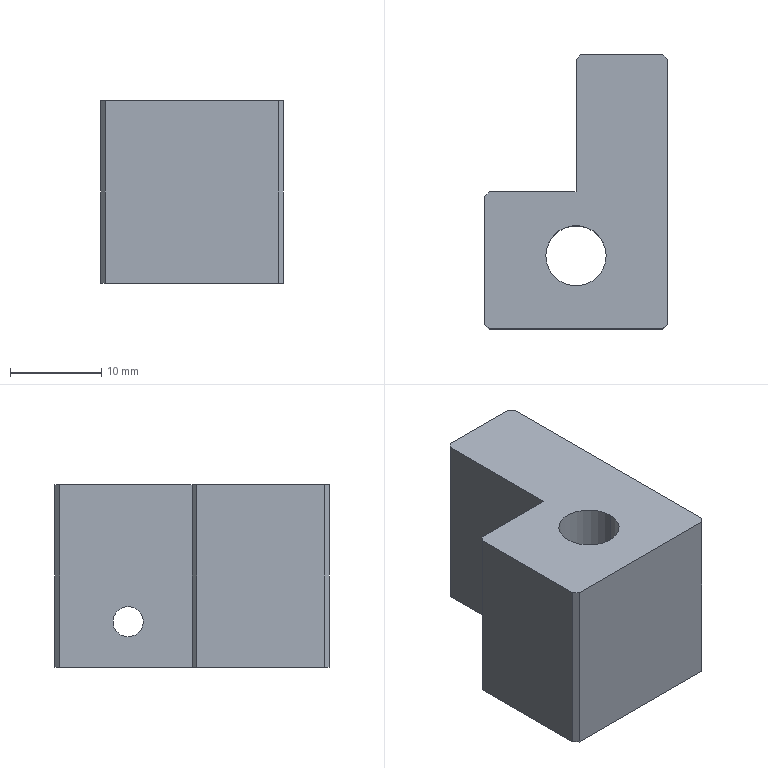Part | SolidWorks | features HoleWzd 2, Chamfer 1, Extrusion 1, ICE 1 | 1 solid | 20 faces | box 20 x 30 x 20 mm | volume 7804 mm3 | plane 14 | cylinder 6 | commonest cylinder face diameters 3.3 x2 6.6 x2 11 x2
STEP:
#1=CARTESIAN_POINT('',(10.,7.,3.35));
#2=VERTEX_POINT('',#1);
#3=CARTESIAN_POINT('',(10.,7.,6.65));
#4=VERTEX_POINT('',#3);
#5=CARTESIAN_POINT('',(10.,7.,5.));
#6=DIRECTION('',(-1.,0.,0.));
#7=DIRECTION('',(0.,0.,1.));
#8=AXIS2_PLACEMENT_3D('',#5,#6,#7);
#9=CIRCLE('',#8,1.65);
#10=EDGE_CURVE('',#2,#4,#9,.T.);
#11=ORIENTED_EDGE('',*,*,#10,.F.);
#12=CARTESIAN_POINT('',(0.,7.,3.35));
#13=VERTEX_POINT('',#12);
#14=CARTESIAN_POINT('',(0.,7.,3.35));
#15=DIRECTION('',(-1.,0.,0.));
#16=VECTOR('',#15,1000.);
#17=LINE('',#14,#16);
#18=EDGE_CURVE('',#2,#13,#17,.T.);
#19=ORIENTED_EDGE('',*,*,#18,.T.);
#20=CARTESIAN_POINT('',(0.,7.,6.65));
#21=VERTEX_POINT('',#20);
#22=CARTESIAN_POINT('',(0.,7.,5.));
#23=DIRECTION('',(-1.,0.,0.));
#24=DIRECTION('',(0.,0.,1.));
#25=AXIS2_PLACEMENT_3D('',#22,#23,#24);
#26=CIRCLE('',#25,1.65);
#27=EDGE_CURVE('',#13,#21,#26,.T.);
#28=ORIENTED_EDGE('',*,*,#27,.T.);
#29=CARTESIAN_POINT('',(0.,7.,6.65));
#30=DIRECTION('',(-1.,0.,0.));
#31=VECTOR('',#30,1000.);
#32=LINE('',#29,#31);
#33=EDGE_CURVE('',#4,#21,#32,.T.);
#34=ORIENTED_EDGE('',*,*,#33,.F.);
#35=EDGE_LOOP('',(#11,#19,#28,#34));
#36=FACE_OUTER_BOUND('',#35,.T.);
#37=CARTESIAN_POINT('',(0.,7.,5.));
#38=DIRECTION('',(-1.,0.,0.));
#39=DIRECTION('',(0.,0.,1.));
#40=AXIS2_PLACEMENT_3D('',#37,#38,#39);
#41=CYLINDRICAL_SURFACE('',#40,1.65);
#42=ADVANCED_FACE('',(#36),#41,.F.);
#43=CARTESIAN_POINT('',(5.5,-7.,6.8));
#44=VERTEX_POINT('',#43);
#45=CARTESIAN_POINT('',(-5.5,-7.,6.8));
#46=VERTEX_POINT('',#45);
#47=CARTESIAN_POINT('',(0.,-7.,6.8));
#48=DIRECTION('',(0.,0.,-1.));
#49=DIRECTION('',(-1.,0.,0.));
#50=AXIS2_PLACEMENT_3D('',#47,#48,#49);
#51=CIRCLE('',#50,5.5);
#52=EDGE_CURVE('',#44,#46,#51,.T.);
#53=ORIENTED_EDGE('',*,*,#52,.F.);
#54=CARTESIAN_POINT('',(5.5,-7.,0.));
#55=VERTEX_POINT('',#54);
#56=CARTESIAN_POINT('',(5.5,-7.,0.));
#57=DIRECTION('',(0.,0.,-1.));
#58=VECTOR('',#57,1000.);
#59=LINE('',#56,#58);
#60=EDGE_CURVE('',#44,#55,#59,.T.);
#61=ORIENTED_EDGE('',*,*,#60,.T.);
#62=CARTESIAN_POINT('',(-5.5,-7.,0.));
#63=VERTEX_POINT('',#62);
#64=CARTESIAN_POINT('',(0.,-7.,0.));
#65=DIRECTION('',(0.,0.,-1.));
#66=DIRECTION('',(-1.,0.,0.));
#67=AXIS2_PLACEMENT_3D('',#64,#65,#66);
#68=CIRCLE('',#67,5.5);
#69=EDGE_CURVE('',#55,#63,#68,.T.);
#70=ORIENTED_EDGE('',*,*,#69,.T.);
#71=CARTESIAN_POINT('',(-5.5,-7.,0.));
#72=DIRECTION('',(0.,0.,-1.));
#73=VECTOR('',#72,1000.);
#74=LINE('',#71,#73);
#75=EDGE_CURVE('',#46,#63,#74,.T.);
#76=ORIENTED_EDGE('',*,*,#75,.F.);
#77=EDGE_LOOP('',(#53,#61,#70,#76));
#78=FACE_OUTER_BOUND('',#77,.T.);
#79=CARTESIAN_POINT('',(0.,-7.,0.));
#80=DIRECTION('',(0.,0.,-1.));
#81=DIRECTION('',(-1.,0.,0.));
#82=AXIS2_PLACEMENT_3D('',#79,#80,#81);
#83=CYLINDRICAL_SURFACE('',#82,5.5);
#84=ADVANCED_FACE('',(#78),#83,.F.);
#85=CARTESIAN_POINT('',(3.3,-7.,20.));
#86=VERTEX_POINT('',#85);
#87=CARTESIAN_POINT('',(-3.3,-7.,20.));
#88=VERTEX_POINT('',#87);
#89=CARTESIAN_POINT('',(0.,-7.,20.));
#90=DIRECTION('',(0.,0.,-1.));
#91=DIRECTION('',(-1.,0.,0.));
#92=AXIS2_PLACEMENT_3D('',#89,#90,#91);
#93=CIRCLE('',#92,3.3);
#94=EDGE_CURVE('',#86,#88,#93,.T.);
#95=ORIENTED_EDGE('',*,*,#94,.F.);
#96=CARTESIAN_POINT('',(3.3,-7.,6.8));
#97=VERTEX_POINT('',#96);
#98=CARTESIAN_POINT('',(3.3,-7.,0.));
#99=DIRECTION('',(0.,0.,-1.));
#100=VECTOR('',#99,1000.);
#101=LINE('',#98,#100);
#102=EDGE_CURVE('',#86,#97,#101,.T.);
#103=ORIENTED_EDGE('',*,*,#102,.T.);
#104=CARTESIAN_POINT('',(-3.3,-7.,6.8));
#105=VERTEX_POINT('',#104);
#106=CARTESIAN_POINT('',(0.,-7.,6.8));
#107=DIRECTION('',(0.,0.,-1.));
#108=DIRECTION('',(-1.,0.,0.));
#109=AXIS2_PLACEMENT_3D('',#106,#107,#108);
#110=CIRCLE('',#109,3.3);
#111=EDGE_CURVE('',#97,#105,#110,.T.);
#112=ORIENTED_EDGE('',*,*,#111,.T.);
#113=CARTESIAN_POINT('',(-3.3,-7.,0.));
#114=DIRECTION('',(0.,0.,-1.));
#115=VECTOR('',#114,1000.);
#116=LINE('',#113,#115);
#117=EDGE_CURVE('',#88,#105,#116,.T.);
#118=ORIENTED_EDGE('',*,*,#117,.F.);
#119=EDGE_LOOP('',(#95,#103,#112,#118));
#120=FACE_OUTER_BOUND('',#119,.T.);
#121=CARTESIAN_POINT('',(0.,-7.,0.));
#122=DIRECTION('',(0.,0.,-1.));
#123=DIRECTION('',(-1.,0.,0.));
#124=AXIS2_PLACEMENT_3D('',#121,#122,#123);
#125=CYLINDRICAL_SURFACE('',#124,3.3);
#126=ADVANCED_FACE('',(#120),#125,.F.);
#127=CARTESIAN_POINT('',(10.,7.,5.));
#128=DIRECTION('',(-1.,0.,0.));
#129=DIRECTION('',(0.,0.,1.));
#130=AXIS2_PLACEMENT_3D('',#127,#128,#129);
#131=CIRCLE('',#130,1.65);
#132=EDGE_CURVE('',#4,#2,#131,.T.);
#133=ORIENTED_EDGE('',*,*,#132,.T.);
#134=ORIENTED_EDGE('',*,*,#10,.T.);
#135=EDGE_LOOP('',(#133,#134));
#136=FACE_BOUND('',#135,.T.);
#137=CARTESIAN_POINT('',(10.,-14.5,0.));
#138=VERTEX_POINT('',#137);
#139=CARTESIAN_POINT('',(10.,14.5,0.));
#140=VERTEX_POINT('',#139);
#141=CARTESIAN_POINT('',(10.,15.,0.));
#142=DIRECTION('',(0.,1.,0.));
#143=VECTOR('',#142,1000.);
#144=LINE('',#141,#143);
#145=EDGE_CURVE('',#138,#140,#144,.T.);
#146=ORIENTED_EDGE('',*,*,#145,.T.);
#147=CARTESIAN_POINT('',(10.,14.5,20.));
#148=VERTEX_POINT('',#147);
#149=CARTESIAN_POINT('',(10.,14.5,20.));
#150=DIRECTION('',(0.,0.,1.));
#151=VECTOR('',#150,1000.);
#152=LINE('',#149,#151);
#153=EDGE_CURVE('',#140,#148,#152,.T.);
#154=ORIENTED_EDGE('',*,*,#153,.T.);
#155=CARTESIAN_POINT('',(10.,-14.5,20.));
#156=VERTEX_POINT('',#155);
#157=CARTESIAN_POINT('',(10.,15.,20.));
#158=DIRECTION('',(0.,1.,0.));
#159=VECTOR('',#158,1000.);
#160=LINE('',#157,#159);
#161=EDGE_CURVE('',#156,#148,#160,.T.);
#162=ORIENTED_EDGE('',*,*,#161,.F.);
#163=CARTESIAN_POINT('',(10.,-14.5,20.));
#164=DIRECTION('',(0.,0.,-1.));
#165=VECTOR('',#164,1000.);
#166=LINE('',#163,#165);
#167=EDGE_CURVE('',#156,#138,#166,.T.);
#168=ORIENTED_EDGE('',*,*,#167,.T.);
#169=EDGE_LOOP('',(#146,#154,#162,#168));
#170=FACE_OUTER_BOUND('',#169,.T.);
#171=CARTESIAN_POINT('',(10.,15.,20.));
#172=DIRECTION('',(-1.,0.,0.));
#173=DIRECTION('',(0.,-1.,0.));
#174=AXIS2_PLACEMENT_3D('',#171,#172,#173);
#175=PLANE('',#174);
#176=ADVANCED_FACE('',(#136,#170),#175,.F.);
#177=CARTESIAN_POINT('',(9.5,15.,20.));
#178=VERTEX_POINT('',#177);
#179=CARTESIAN_POINT('',(0.5,15.,20.));
#180=VERTEX_POINT('',#179);
#181=CARTESIAN_POINT('',(-10.,15.,20.));
#182=DIRECTION('',(-1.,0.,0.));
#183=VECTOR('',#182,1000.);
#184=LINE('',#181,#183);
#185=EDGE_CURVE('',#178,#180,#184,.T.);
#186=ORIENTED_EDGE('',*,*,#185,.F.);
#187=CARTESIAN_POINT('',(9.5,15.,0.));
#188=VERTEX_POINT('',#187);
#189=CARTESIAN_POINT('',(9.5,15.,20.));
#190=DIRECTION('',(0.,0.,-1.));
#191=VECTOR('',#190,1000.);
#192=LINE('',#189,#191);
#193=EDGE_CURVE('',#178,#188,#192,.T.);
#194=ORIENTED_EDGE('',*,*,#193,.T.);
#195=CARTESIAN_POINT('',(0.5,15.,0.));
#196=VERTEX_POINT('',#195);
#197=CARTESIAN_POINT('',(-10.,15.,0.));
#198=DIRECTION('',(-1.,0.,0.));
#199=VECTOR('',#198,1000.);
#200=LINE('',#197,#199);
#201=EDGE_CURVE('',#188,#196,#200,.T.);
#202=ORIENTED_EDGE('',*,*,#201,.T.);
#203=CARTESIAN_POINT('',(0.5,15.,20.));
#204=DIRECTION('',(0.,0.,1.));
#205=VECTOR('',#204,1000.);
#206=LINE('',#203,#205);
#207=EDGE_CURVE('',#196,#180,#206,.T.);
#208=ORIENTED_EDGE('',*,*,#207,.T.);
#209=EDGE_LOOP('',(#186,#194,#202,#208));
#210=FACE_OUTER_BOUND('',#209,.T.);
#211=CARTESIAN_POINT('',(-10.,15.,20.));
#212=DIRECTION('',(0.,-1.,0.));
#213=DIRECTION('',(0.,0.,-1.));
#214=AXIS2_PLACEMENT_3D('',#211,#212,#213);
#215=PLANE('',#214);
#216=ADVANCED_FACE('',(#210),#215,.F.);
#217=CARTESIAN_POINT('',(-10.,-0.5,20.));
#218=VERTEX_POINT('',#217);
#219=CARTESIAN_POINT('',(-10.,-14.5,20.));
#220=VERTEX_POINT('',#219);
#221=CARTESIAN_POINT('',(-10.,15.,20.));
#222=DIRECTION('',(0.,-1.,0.));
#223=VECTOR('',#222,1000.);
#224=LINE('',#221,#223);
#225=EDGE_CURVE('',#218,#220,#224,.T.);
#226=ORIENTED_EDGE('',*,*,#225,.F.);
#227=CARTESIAN_POINT('',(-10.,-0.5,0.));
#228=VERTEX_POINT('',#227);
#229=CARTESIAN_POINT('',(-10.,-0.5,20.));
#230=DIRECTION('',(0.,0.,-1.));
#231=VECTOR('',#230,1000.);
#232=LINE('',#229,#231);
#233=EDGE_CURVE('',#218,#228,#232,.T.);
#234=ORIENTED_EDGE('',*,*,#233,.T.);
#235=CARTESIAN_POINT('',(-10.,-14.5,0.));
#236=VERTEX_POINT('',#235);
#237=CARTESIAN_POINT('',(-10.,15.,0.));
#238=DIRECTION('',(0.,-1.,0.));
#239=VECTOR('',#238,1000.);
#240=LINE('',#237,#239);
#241=EDGE_CURVE('',#228,#236,#240,.T.);
#242=ORIENTED_EDGE('',*,*,#241,.T.);
#243=CARTESIAN_POINT('',(-10.,-14.5,20.));
#244=DIRECTION('',(0.,0.,1.));
#245=VECTOR('',#244,1000.);
#246=LINE('',#243,#245);
#247=EDGE_CURVE('',#236,#220,#246,.T.);
#248=ORIENTED_EDGE('',*,*,#247,.T.);
#249=EDGE_LOOP('',(#226,#234,#242,#248));
#250=FACE_OUTER_BOUND('',#249,.T.);
#251=CARTESIAN_POINT('',(-10.,15.,20.));
#252=DIRECTION('',(1.,0.,0.));
#253=DIRECTION('',(0.,1.,0.));
#254=AXIS2_PLACEMENT_3D('',#251,#252,#253);
#255=PLANE('',#254);
#256=ADVANCED_FACE('',(#250),#255,.F.);
#257=CARTESIAN_POINT('',(-9.5,-15.,20.));
#258=VERTEX_POINT('',#257);
#259=CARTESIAN_POINT('',(9.5,-15.,20.));
#260=VERTEX_POINT('',#259);
#261=CARTESIAN_POINT('',(-10.,-15.,20.));
#262=DIRECTION('',(1.,0.,0.));
#263=VECTOR('',#262,1000.);
#264=LINE('',#261,#263);
#265=EDGE_CURVE('',#258,#260,#264,.T.);
#266=ORIENTED_EDGE('',*,*,#265,.F.);
#267=CARTESIAN_POINT('',(-9.5,-15.,0.));
#268=VERTEX_POINT('',#267);
#269=CARTESIAN_POINT('',(-9.5,-15.,20.));
#270=DIRECTION('',(0.,0.,-1.));
#271=VECTOR('',#270,1000.);
#272=LINE('',#269,#271);
#273=EDGE_CURVE('',#258,#268,#272,.T.);
#274=ORIENTED_EDGE('',*,*,#273,.T.);
#275=CARTESIAN_POINT('',(9.5,-15.,0.));
#276=VERTEX_POINT('',#275);
#277=CARTESIAN_POINT('',(-10.,-15.,0.));
#278=DIRECTION('',(1.,0.,0.));
#279=VECTOR('',#278,1000.);
#280=LINE('',#277,#279);
#281=EDGE_CURVE('',#268,#276,#280,.T.);
#282=ORIENTED_EDGE('',*,*,#281,.T.);
#283=CARTESIAN_POINT('',(9.5,-15.,20.));
#284=DIRECTION('',(0.,0.,1.));
#285=VECTOR('',#284,1000.);
#286=LINE('',#283,#285);
#287=EDGE_CURVE('',#276,#260,#286,.T.);
#288=ORIENTED_EDGE('',*,*,#287,.T.);
#289=EDGE_LOOP('',(#266,#274,#282,#288));
#290=FACE_OUTER_BOUND('',#289,.T.);
#291=CARTESIAN_POINT('',(-10.,-15.,20.));
#292=DIRECTION('',(0.,1.,0.));
#293=DIRECTION('',(0.,0.,1.));
#294=AXIS2_PLACEMENT_3D('',#291,#292,#293);
#295=PLANE('',#294);
#296=ADVANCED_FACE('',(#290),#295,.F.);
#297=ORIENTED_EDGE('',*,*,#161,.T.);
#298=CARTESIAN_POINT('',(24.75,-0.25,20.));
#299=DIRECTION('',(-0.7071,0.7071,0.));
#300=VECTOR('',#299,1000.);
#301=LINE('',#298,#300);
#302=EDGE_CURVE('',#148,#178,#301,.T.);
#303=ORIENTED_EDGE('',*,*,#302,.T.);
#304=ORIENTED_EDGE('',*,*,#185,.T.);
#305=CARTESIAN_POINT('',(0.,14.5,20.));
#306=VERTEX_POINT('',#305);
#307=CARTESIAN_POINT('',(-9.75,4.75,20.));
#308=DIRECTION('',(-0.7071,-0.7071,0.));
#309=VECTOR('',#308,1000.);
#310=LINE('',#307,#309);
#311=EDGE_CURVE('',#180,#306,#310,.T.);
#312=ORIENTED_EDGE('',*,*,#311,.T.);
#313=CARTESIAN_POINT('',(0.,0.,20.));
#314=VERTEX_POINT('',#313);
#315=CARTESIAN_POINT('',(0.,15.,20.));
#316=DIRECTION('',(0.,1.,0.));
#317=VECTOR('',#316,1000.);
#318=LINE('',#315,#317);
#319=EDGE_CURVE('',#314,#306,#318,.T.);
#320=ORIENTED_EDGE('',*,*,#319,.F.);
#321=CARTESIAN_POINT('',(-9.5,0.,20.));
#322=VERTEX_POINT('',#321);
#323=CARTESIAN_POINT('',(-10.,0.,20.));
#324=DIRECTION('',(1.,0.,0.));
#325=VECTOR('',#324,1000.);
#326=LINE('',#323,#325);
#327=EDGE_CURVE('',#322,#314,#326,.T.);
#328=ORIENTED_EDGE('',*,*,#327,.F.);
#329=CARTESIAN_POINT('',(-7.25,2.25,20.));
#330=DIRECTION('',(-0.7071,-0.7071,0.));
#331=VECTOR('',#330,1000.);
#332=LINE('',#329,#331);
#333=EDGE_CURVE('',#322,#218,#332,.T.);
#334=ORIENTED_EDGE('',*,*,#333,.T.);
#335=ORIENTED_EDGE('',*,*,#225,.T.);
#336=CARTESIAN_POINT('',(0.25,-24.75,20.));
#337=DIRECTION('',(0.7071,-0.7071,0.));
#338=VECTOR('',#337,1000.);
#339=LINE('',#336,#338);
#340=EDGE_CURVE('',#220,#258,#339,.T.);
#341=ORIENTED_EDGE('',*,*,#340,.T.);
#342=ORIENTED_EDGE('',*,*,#265,.T.);
#343=CARTESIAN_POINT('',(9.75,-14.75,20.));
#344=DIRECTION('',(0.7071,0.7071,0.));
#345=VECTOR('',#344,1000.);
#346=LINE('',#343,#345);
#347=EDGE_CURVE('',#260,#156,#346,.T.);
#348=ORIENTED_EDGE('',*,*,#347,.T.);
#349=EDGE_LOOP('',(#297,#303,#304,#312,#320,#328,#334,#335,#341,#342,#348));
#350=FACE_OUTER_BOUND('',#349,.T.);
#351=CARTESIAN_POINT('',(0.,-7.,20.));
#352=DIRECTION('',(0.,0.,-1.));
#353=DIRECTION('',(-1.,0.,0.));
#354=AXIS2_PLACEMENT_3D('',#351,#352,#353);
#355=CIRCLE('',#354,3.3);
#356=EDGE_CURVE('',#88,#86,#355,.T.);
#357=ORIENTED_EDGE('',*,*,#356,.T.);
#358=ORIENTED_EDGE('',*,*,#94,.T.);
#359=EDGE_LOOP('',(#357,#358));
#360=FACE_BOUND('',#359,.T.);
#361=CARTESIAN_POINT('',(10.,-15.,20.));
#362=DIRECTION('',(0.,0.,1.));
#363=DIRECTION('',(1.,0.,0.));
#364=AXIS2_PLACEMENT_3D('',#361,#362,#363);
#365=PLANE('',#364);
#366=ADVANCED_FACE('',(#350,#360),#365,.T.);
#367=CARTESIAN_POINT('',(0.,-7.,0.));
#368=DIRECTION('',(0.,0.,-1.));
#369=DIRECTION('',(-1.,0.,0.));
#370=AXIS2_PLACEMENT_3D('',#367,#368,#369);
#371=CIRCLE('',#370,5.5);
#372=EDGE_CURVE('',#63,#55,#371,.T.);
#373=ORIENTED_EDGE('',*,*,#372,.F.);
#374=ORIENTED_EDGE('',*,*,#69,.F.);
#375=EDGE_LOOP('',(#373,#374));
#376=FACE_BOUND('',#375,.T.);
#377=ORIENTED_EDGE('',*,*,#201,.F.);
#378=CARTESIAN_POINT('',(9.5,15.,0.));
#379=DIRECTION('',(0.7071,-0.7071,0.));
#380=VECTOR('',#379,1000.);
#381=LINE('',#378,#380);
#382=EDGE_CURVE('',#188,#140,#381,.T.);
#383=ORIENTED_EDGE('',*,*,#382,.T.);
#384=ORIENTED_EDGE('',*,*,#145,.F.);
#385=CARTESIAN_POINT('',(10.,-14.5,0.));
#386=DIRECTION('',(-0.7071,-0.7071,0.));
#387=VECTOR('',#386,1000.);
#388=LINE('',#385,#387);
#389=EDGE_CURVE('',#138,#276,#388,.T.);
#390=ORIENTED_EDGE('',*,*,#389,.T.);
#391=ORIENTED_EDGE('',*,*,#281,.F.);
#392=CARTESIAN_POINT('',(-9.5,-15.,0.));
#393=DIRECTION('',(-0.7071,0.7071,0.));
#394=VECTOR('',#393,1000.);
#395=LINE('',#392,#394);
#396=EDGE_CURVE('',#268,#236,#395,.T.);
#397=ORIENTED_EDGE('',*,*,#396,.T.);
#398=ORIENTED_EDGE('',*,*,#241,.F.);
#399=CARTESIAN_POINT('',(-9.5,0.,0.));
#400=VERTEX_POINT('',#399);
#401=CARTESIAN_POINT('',(-9.5,0.,0.));
#402=DIRECTION('',(0.7071,0.7071,0.));
#403=VECTOR('',#402,1000.);
#404=LINE('',#401,#403);
#405=EDGE_CURVE('',#228,#400,#404,.T.);
#406=ORIENTED_EDGE('',*,*,#405,.T.);
#407=CARTESIAN_POINT('',(0.,0.,0.));
#408=VERTEX_POINT('',#407);
#409=CARTESIAN_POINT('',(-10.,0.,0.));
#410=DIRECTION('',(1.,0.,0.));
#411=VECTOR('',#410,1000.);
#412=LINE('',#409,#411);
#413=EDGE_CURVE('',#400,#408,#412,.T.);
#414=ORIENTED_EDGE('',*,*,#413,.T.);
#415=CARTESIAN_POINT('',(0.,14.5,0.));
#416=VERTEX_POINT('',#415);
#417=CARTESIAN_POINT('',(0.,15.,0.));
#418=DIRECTION('',(0.,1.,0.));
#419=VECTOR('',#418,1000.);
#420=LINE('',#417,#419);
#421=EDGE_CURVE('',#408,#416,#420,.T.);
#422=ORIENTED_EDGE('',*,*,#421,.T.);
#423=CARTESIAN_POINT('',(0.5,15.,0.));
#424=DIRECTION('',(0.7071,0.7071,0.));
#425=VECTOR('',#424,1000.);
#426=LINE('',#423,#425);
#427=EDGE_CURVE('',#416,#196,#426,.T.);
#428=ORIENTED_EDGE('',*,*,#427,.T.);
#429=EDGE_LOOP('',(#377,#383,#384,#390,#391,#397,#398,#406,#414,#422,#428));
#430=FACE_OUTER_BOUND('',#429,.T.);
#431=CARTESIAN_POINT('',(10.,-15.,0.));
#432=DIRECTION('',(0.,0.,1.));
#433=DIRECTION('',(1.,0.,0.));
#434=AXIS2_PLACEMENT_3D('',#431,#432,#433);
#435=PLANE('',#434);
#436=ADVANCED_FACE('',(#376,#430),#435,.F.);
#437=ORIENTED_EDGE('',*,*,#102,.F.);
#438=ORIENTED_EDGE('',*,*,#356,.F.);
#439=ORIENTED_EDGE('',*,*,#117,.T.);
#440=CARTESIAN_POINT('',(0.,-7.,6.8));
#441=DIRECTION('',(0.,0.,-1.));
#442=DIRECTION('',(-1.,0.,0.));
#443=AXIS2_PLACEMENT_3D('',#440,#441,#442);
#444=CIRCLE('',#443,3.3);
#445=EDGE_CURVE('',#105,#97,#444,.T.);
#446=ORIENTED_EDGE('',*,*,#445,.T.);
#447=EDGE_LOOP('',(#437,#438,#439,#446));
#448=FACE_OUTER_BOUND('',#447,.T.);
#449=CARTESIAN_POINT('',(0.,-7.,0.));
#450=DIRECTION('',(0.,0.,-1.));
#451=DIRECTION('',(-1.,0.,0.));
#452=AXIS2_PLACEMENT_3D('',#449,#450,#451);
#453=CYLINDRICAL_SURFACE('',#452,3.3);
#454=ADVANCED_FACE('',(#448),#453,.F.);
#455=ORIENTED_EDGE('',*,*,#445,.F.);
#456=ORIENTED_EDGE('',*,*,#111,.F.);
#457=EDGE_LOOP('',(#455,#456));
#458=FACE_BOUND('',#457,.T.);
#459=CARTESIAN_POINT('',(0.,-7.,6.8));
#460=DIRECTION('',(0.,0.,-1.));
#461=DIRECTION('',(-1.,0.,0.));
#462=AXIS2_PLACEMENT_3D('',#459,#460,#461);
#463=CIRCLE('',#462,5.5);
#464=EDGE_CURVE('',#46,#44,#463,.T.);
#465=ORIENTED_EDGE('',*,*,#464,.T.);
#466=ORIENTED_EDGE('',*,*,#52,.T.);
#467=EDGE_LOOP('',(#465,#466));
#468=FACE_OUTER_BOUND('',#467,.T.);
#469=CARTESIAN_POINT('',(3.3,-7.,6.8));
#470=DIRECTION('',(0.,0.,1.));
#471=DIRECTION('',(1.,0.,0.));
#472=AXIS2_PLACEMENT_3D('',#469,#470,#471);
#473=PLANE('',#472);
#474=ADVANCED_FACE('',(#458,#468),#473,.F.);
#475=ORIENTED_EDGE('',*,*,#60,.F.);
#476=ORIENTED_EDGE('',*,*,#464,.F.);
#477=ORIENTED_EDGE('',*,*,#75,.T.);
#478=ORIENTED_EDGE('',*,*,#372,.T.);
#479=EDGE_LOOP('',(#475,#476,#477,#478));
#480=FACE_OUTER_BOUND('',#479,.T.);
#481=CARTESIAN_POINT('',(0.,-7.,0.));
#482=DIRECTION('',(0.,0.,-1.));
#483=DIRECTION('',(-1.,0.,0.));
#484=AXIS2_PLACEMENT_3D('',#481,#482,#483);
#485=CYLINDRICAL_SURFACE('',#484,5.5);
#486=ADVANCED_FACE('',(#480),#485,.F.);
#487=CARTESIAN_POINT('',(0.,7.,5.));
#488=DIRECTION('',(-1.,0.,0.));
#489=DIRECTION('',(0.,0.,1.));
#490=AXIS2_PLACEMENT_3D('',#487,#488,#489);
#491=CIRCLE('',#490,1.65);
#492=EDGE_CURVE('',#21,#13,#491,.T.);
#493=ORIENTED_EDGE('',*,*,#492,.F.);
#494=ORIENTED_EDGE('',*,*,#27,.F.);
#495=EDGE_LOOP('',(#493,#494));
#496=FACE_BOUND('',#495,.T.);
#497=ORIENTED_EDGE('',*,*,#319,.T.);
#498=CARTESIAN_POINT('',(0.,14.5,0.));
#499=DIRECTION('',(0.,0.,-1.));
#500=VECTOR('',#499,1000.);
#501=LINE('',#498,#500);
#502=EDGE_CURVE('',#306,#416,#501,.T.);
#503=ORIENTED_EDGE('',*,*,#502,.T.);
#504=ORIENTED_EDGE('',*,*,#421,.F.);
#505=CARTESIAN_POINT('',(0.,0.,0.));
#506=DIRECTION('',(0.,0.,1.));
#507=VECTOR('',#506,1000.);
#508=LINE('',#505,#507);
#509=EDGE_CURVE('',#408,#314,#508,.T.);
#510=ORIENTED_EDGE('',*,*,#509,.T.);
#511=EDGE_LOOP('',(#497,#503,#504,#510));
#512=FACE_OUTER_BOUND('',#511,.T.);
#513=CARTESIAN_POINT('',(0.,15.,0.));
#514=DIRECTION('',(1.,0.,0.));
#515=DIRECTION('',(0.,1.,0.));
#516=AXIS2_PLACEMENT_3D('',#513,#514,#515);
#517=PLANE('',#516);
#518=ADVANCED_FACE('',(#496,#512),#517,.F.);
#519=ORIENTED_EDGE('',*,*,#413,.F.);
#520=CARTESIAN_POINT('',(-9.5,0.,0.));
#521=DIRECTION('',(0.,0.,1.));
#522=VECTOR('',#521,1000.);
#523=LINE('',#520,#522);
#524=EDGE_CURVE('',#400,#322,#523,.T.);
#525=ORIENTED_EDGE('',*,*,#524,.T.);
#526=ORIENTED_EDGE('',*,*,#327,.T.);
#527=ORIENTED_EDGE('',*,*,#509,.F.);
#528=EDGE_LOOP('',(#519,#525,#526,#527));
#529=FACE_OUTER_BOUND('',#528,.T.);
#530=CARTESIAN_POINT('',(-10.,0.,0.));
#531=DIRECTION('',(0.,-1.,0.));
#532=DIRECTION('',(1.,0.,0.));
#533=AXIS2_PLACEMENT_3D('',#530,#531,#532);
#534=PLANE('',#533);
#535=ADVANCED_FACE('',(#529),#534,.F.);
#536=ORIENTED_EDGE('',*,*,#18,.F.);
#537=ORIENTED_EDGE('',*,*,#132,.F.);
#538=ORIENTED_EDGE('',*,*,#33,.T.);
#539=ORIENTED_EDGE('',*,*,#492,.T.);
#540=EDGE_LOOP('',(#536,#537,#538,#539));
#541=FACE_OUTER_BOUND('',#540,.T.);
#542=CARTESIAN_POINT('',(0.,7.,5.));
#543=DIRECTION('',(-1.,0.,0.));
#544=DIRECTION('',(0.,0.,1.));
#545=AXIS2_PLACEMENT_3D('',#542,#543,#544);
#546=CYLINDRICAL_SURFACE('',#545,1.65);
#547=ADVANCED_FACE('',(#541),#546,.F.);
#548=ORIENTED_EDGE('',*,*,#302,.F.);
#549=ORIENTED_EDGE('',*,*,#153,.F.);
#550=ORIENTED_EDGE('',*,*,#382,.F.);
#551=ORIENTED_EDGE('',*,*,#193,.F.);
#552=EDGE_LOOP('',(#548,#549,#550,#551));
#553=FACE_OUTER_BOUND('',#552,.T.);
#554=CARTESIAN_POINT('',(9.5,15.,20.));
#555=DIRECTION('',(-0.7071,-0.7071,0.));
#556=DIRECTION('',(0.7071,-0.7071,0.));
#557=AXIS2_PLACEMENT_3D('',#554,#555,#556);
#558=PLANE('',#557);
#559=ADVANCED_FACE('',(#553),#558,.F.);
#560=ORIENTED_EDGE('',*,*,#427,.F.);
#561=ORIENTED_EDGE('',*,*,#502,.F.);
#562=ORIENTED_EDGE('',*,*,#311,.F.);
#563=ORIENTED_EDGE('',*,*,#207,.F.);
#564=EDGE_LOOP('',(#560,#561,#562,#563));
#565=FACE_OUTER_BOUND('',#564,.T.);
#566=CARTESIAN_POINT('',(0.5,15.,20.));
#567=DIRECTION('',(0.7071,-0.7071,0.));
#568=DIRECTION('',(0.7071,0.7071,0.));
#569=AXIS2_PLACEMENT_3D('',#566,#567,#568);
#570=PLANE('',#569);
#571=ADVANCED_FACE('',(#565),#570,.F.);
#572=ORIENTED_EDGE('',*,*,#405,.F.);
#573=ORIENTED_EDGE('',*,*,#233,.F.);
#574=ORIENTED_EDGE('',*,*,#333,.F.);
#575=ORIENTED_EDGE('',*,*,#524,.F.);
#576=EDGE_LOOP('',(#572,#573,#574,#575));
#577=FACE_OUTER_BOUND('',#576,.T.);
#578=CARTESIAN_POINT('',(-9.5,0.,0.));
#579=DIRECTION('',(0.7071,-0.7071,0.));
#580=DIRECTION('',(0.7071,0.7071,0.));
#581=AXIS2_PLACEMENT_3D('',#578,#579,#580);
#582=PLANE('',#581);
#583=ADVANCED_FACE('',(#577),#582,.F.);
#584=ORIENTED_EDGE('',*,*,#340,.F.);
#585=ORIENTED_EDGE('',*,*,#247,.F.);
#586=ORIENTED_EDGE('',*,*,#396,.F.);
#587=ORIENTED_EDGE('',*,*,#273,.F.);
#588=EDGE_LOOP('',(#584,#585,#586,#587));
#589=FACE_OUTER_BOUND('',#588,.T.);
#590=CARTESIAN_POINT('',(-9.5,-15.,20.));
#591=DIRECTION('',(0.7071,0.7071,0.));
#592=DIRECTION('',(-0.7071,0.7071,0.));
#593=AXIS2_PLACEMENT_3D('',#590,#591,#592);
#594=PLANE('',#593);
#595=ADVANCED_FACE('',(#589),#594,.F.);
#596=ORIENTED_EDGE('',*,*,#347,.F.);
#597=ORIENTED_EDGE('',*,*,#287,.F.);
#598=ORIENTED_EDGE('',*,*,#389,.F.);
#599=ORIENTED_EDGE('',*,*,#167,.F.);
#600=EDGE_LOOP('',(#596,#597,#598,#599));
#601=FACE_OUTER_BOUND('',#600,.T.);
#602=CARTESIAN_POINT('',(10.,-14.5,20.));
#603=DIRECTION('',(-0.7071,0.7071,0.));
#604=DIRECTION('',(-0.7071,-0.7071,0.));
#605=AXIS2_PLACEMENT_3D('',#602,#603,#604);
#606=PLANE('',#605);
#607=ADVANCED_FACE('',(#601),#606,.F.);
#608=CLOSED_SHELL('',(#42,#84,#126,#176,#216,#256,#296,#366,#436,#454,#474,#486,#518,#535,#547,#559,#571,#583,#595,#607));
#609=MANIFOLD_SOLID_BREP('',#608);
#610=CARTESIAN_POINT('',(0.,0.,0.));
#611=DIRECTION('',(0.,0.,1.));
#612=DIRECTION('',(1.,0.,0.));
#613=AXIS2_PLACEMENT_3D('',#610,#611,#612);
#614=(LENGTH_UNIT()NAMED_UNIT(*)SI_UNIT(.MILLI.,.METRE.));
#615=UNCERTAINTY_MEASURE_WITH_UNIT(LENGTH_MEASURE(0.00001),#614,'','');
#616=(NAMED_UNIT(*)PLANE_ANGLE_UNIT()SI_UNIT($,.RADIAN.));
#617=(NAMED_UNIT(*)SI_UNIT($,.STERADIAN.)SOLID_ANGLE_UNIT());
#618=(GEOMETRIC_REPRESENTATION_CONTEXT(3)GLOBAL_UNCERTAINTY_ASSIGNED_CONTEXT((#615))GLOBAL_UNIT_ASSIGNED_CONTEXT((#614,#616,#617))REPRESENTATION_CONTEXT('',''));
#619=ADVANCED_BREP_SHAPE_REPRESENTATION('',(#609,#613),#618);